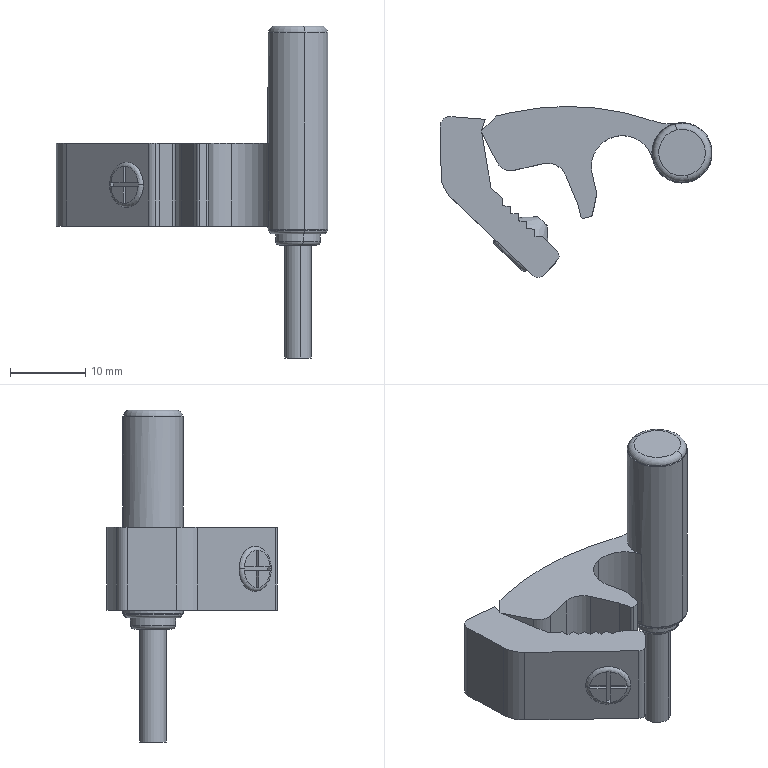Part | SolidWorks | features BaseBody 1 | 1 solid | 97 faces | box 36.145 x 22.709 x 44.1 mm | volume 4669 mm3 | plane 55 | cylinder 26 | torus 12 | cone 4 | commonest cylinder face diameters 6 x8 2 x3 8 x3 0.6 x2 2.7 x2 3.5 x2